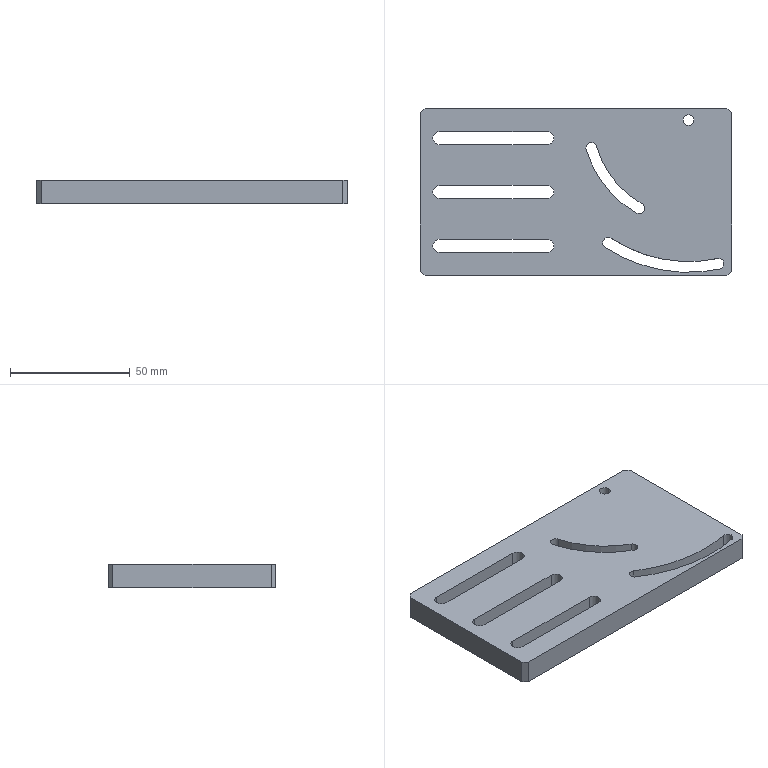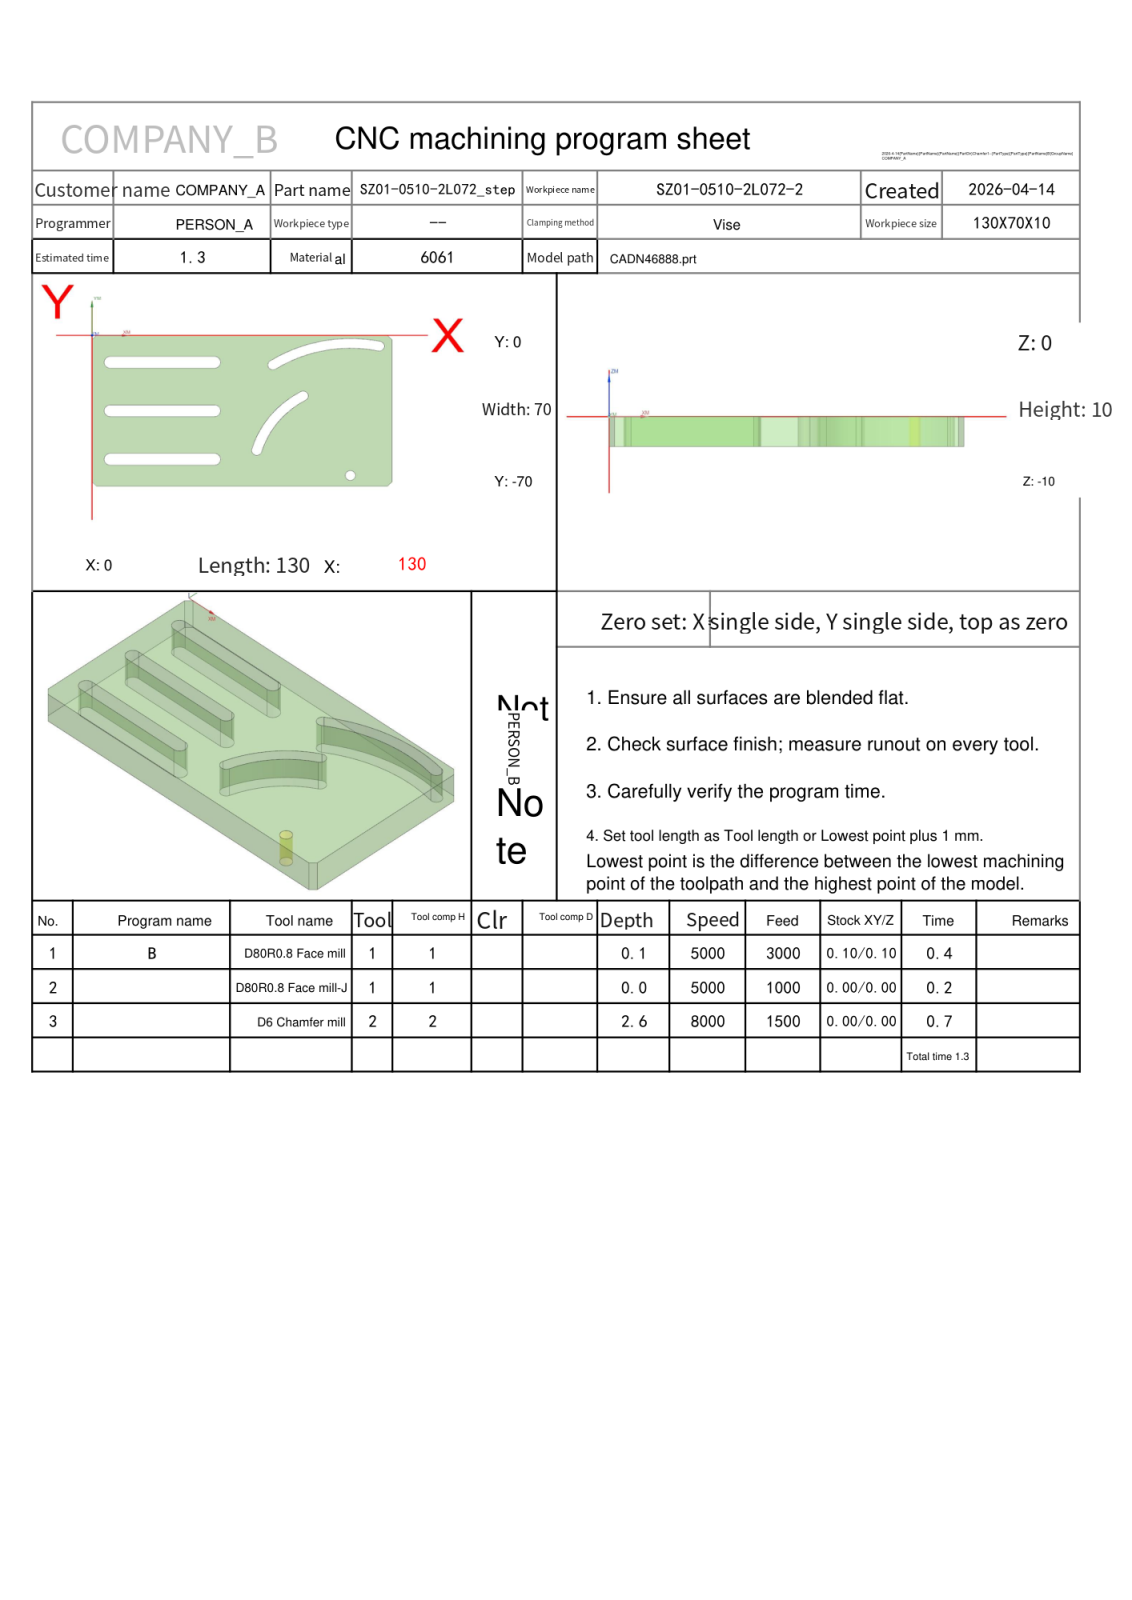NC program | NX | posted by the shop | part box 130 x 70 x 10 mm
Whole program:
%
O0001
(Machine time: 1.90 MIN)
(===Total Tool:2===)
(T1=D80R0.8 Face mill D=80.  R=0.8  D-  H01 Z=0.    )
(T2=D6 Chamfer mill   D=6.   R=0.   D-  H02 Z=-2.55 )
G80 G90 G17 G49 G40
G91 G28 Z0
M01
N1 T01 M06
(D80R0.8 Face mill  D=80. R=0.8 H=01 ce=0.10 di=0.10)
G00 G90 G54 X182.097 Y-35. M03 S5000
G43 H01 Z20.
M08
Z3.375
G01 Z1.375 F3000.
X170.097
X-40.097
X-52.097
Z3.375
G00 X182.097
Z2.95
G01 Z.95
X170.097
X-40.097
X-52.097
Z2.95
G00 X182.097
Z2.525
G01 Z.525
X170.097
X-40.097
X-52.097
Z2.525
G00 X182.097
Z2.1
G01 Z.1
X170.097
X-40.097
X-52.097
Z2.1
G00 Z20.
G91 G28 Z0.0
M05
M09
G91 G28 Z0.0
M01
N2 T01 M06
(D80R0.8 Face mill-J  D=80. R=0.8 H=01 ce=0.00 di=0.00)
G00 G90 G54 X181.999 Y-35. M03 S5000
G43 H01 Z20.
M08
Z2.
G01 Z0.0 F1000.
X169.999
X-39.999
X-51.999
Z2.
G00 Z20.
G91 G28 Z0.0
M05
M09
G91 G28 Z0.0
M01
N3 T02 M06
(D6 Chamfer mill  D=6. R=0. H=02 ce=0.00 di=0.00)
G00 G90 G54 X112. Y-65. M03 S8000
G43 H02 Z20.
M08
G98 G81 X112. Y-65. Z-2.55 R3. F1000.
G80
G00 Z20.
G00 G90 X64.614 Y1.227 M03 S6500
Z20.
Z.172
G01 Z-1.2 F1500.
G03 X64.9 Y1.027 I1.286 J1.532
G01 X64.946 Y.997
X65. Y1.
X128.
X128.259 Y.966
X128.5 Y.866
X128.707 Y.707
X130.707 Y-1.293
X130.866 Y-1.5
X130.966 Y-1.741
X131. Y-2.
Y-68.
X130.966 Y-68.259
X130.866 Y-68.5
X130.707 Y-68.707
X128.707 Y-70.707
X128.5 Y-70.866
X128.259 Y-70.966
X128. Y-71.
X2.
X1.741 Y-70.966
X1.5 Y-70.866
X1.293 Y-70.707
X-.707 Y-68.707
X-.866 Y-68.5
X-.966 Y-68.259
X-1. Y-68.
Y-2.
X-.966 Y-1.741
X-.866 Y-1.5
X-.707 Y-1.293
X1.293 Y.707
X1.5 Y.866
X1.741 Y.966
X2. Y1.
X65.
X65.054 Y.997
X65.1 Y1.027
G03 X65.386 Y1.227 I-1. J1.732
G01 Z.172
G00 Z10.
X113.065 Y-65.407
Z.294
G01 Z-1.2
G03 X113.234 Y-65.102 I-1.658 J1.118
G01 X113.259 Y-65.054
X113.25 Y-65.
G03 X112. Y-63.75 I-1.25 J0.0
X110.75 Y-65. I0.0 J-1.25
X112. Y-66.25 I1.25 J0.0
X113.223 Y-65.26 I0.0 J1.25
G01 X113.25 Y-65.
X113.259 Y-64.946
X113.234 Y-64.898
G03 X113.065 Y-64.593 I-1.827 J-.813
G01 Z.294
G00 Z10.
X78.375 Y-37.807
Z.189
G01 Z-1.2
G03 X78.042 Y-37.913 I.439 J-1.951
G01 X77.991 Y-37.932
X77.96 Y-37.977
G03 X70.21 Y-53.06 I34.04 J-27.023
X70.162 Y-53.403 I1.202 J-.343
X71.412 Y-54.653 I1.25 J0.0
X72.614 Y-53.747 I0.0 J1.25
G02 X92.107 Y-29.193 I39.386 J-11.253
G03 X92.75 Y-28.1 I-.607 J1.093
X91.5 Y-26.85 I-1.25 J0.0
X90.893 Y-27.007 I0.0 J-1.25
X77.96 Y-37.977 I21.107 J-37.993
G01 X77.924 Y-38.017
X77.917 Y-38.071
G03 X77.89 Y-38.403 I1.972 J-.333
G01 Y-38.418
Z.189
G00 Z10.
X100.778 Y-3.699
Z.188
G01 Z-1.2
G03 X100.458 Y-3.561 I-.947 J-1.762
G01 X100.407 Y-3.542
X100.355 Y-3.556
G03 X77.727 Y-12.689 I11.645 J-61.444
X77.162 Y-13.735 I.685 J-1.046
X78.412 Y-14.985 I1.25 J0.0
X79.097 Y-14.78 I0.0 J1.25
G02 X112. Y-4.962 I32.903 J-50.22
X124.245 Y-6.224 I0.0 J-60.038
G03 X124.5 Y-6.25 I.255 J1.224
X125.75 Y-5. I0.0 J1.25
X124.755 Y-3.776 I-1.25 J0.0
X112. Y-2.462 I-12.755 J-61.224
X100.355 Y-3.556 I0.0 J-62.538
G01 X100.301 Y-3.562
X100.261 Y-3.599
G03 X100.013 Y-3.844 I1.278 J-1.539
G01 Z.188
G00 Z10.
X30.886 Y-10.977
Z.172
G01 Z-1.2
G03 X30.6 Y-10.777 I-1.286 J-1.532
G01 X30.554 Y-10.747
X30.5 Y-10.75
X8.
G03 X6.25 Y-12.5 I0.0 J-1.75
X8. Y-14.25 I1.75 J0.0
G01 X53.
G03 X54.75 Y-12.5 I0.0 J1.75
X53. Y-10.75 I-1.75 J0.0
G01 X30.5
X30.446 Y-10.747
X30.4 Y-10.777
G03 X30.114 Y-10.977 I1. J-1.732
G01 Z.172
G00 Z10.
Y-36.523
Z.172
G01 Z-1.2
G03 X30.4 Y-36.723 I1.286 J1.532
G01 X30.446 Y-36.753
X30.5 Y-36.75
X53.
G03 X54.75 Y-35. I0.0 J1.75
X53. Y-33.25 I-1.75 J0.0
G01 X8.
G03 X6.25 Y-35. I0.0 J-1.75
X8. Y-36.75 I1.75 J0.0
G01 X30.5
X30.554 Y-36.753
X30.6 Y-36.723
G03 X30.886 Y-36.523 I-1. J1.732
G01 Z.172
G00 Z10.
X30.114 Y-59.023
Z.172
G01 Z-1.2
G03 X30.4 Y-59.223 I1.286 J1.532
G01 X30.446 Y-59.253
X30.5 Y-59.25
X53.
G03 X54.75 Y-57.5 I0.0 J1.75
X53. Y-55.75 I-1.75 J0.0
G01 X8.
G03 X6.25 Y-57.5 I0.0 J-1.75
X8. Y-59.25 I1.75 J0.0
G01 X30.5
X30.554 Y-59.253
X30.6 Y-59.223
G03 X30.886 Y-59.023 I-1. J1.732
G01 Z.172
G00 Z20.
M05
M09
G91 G28 Z0.0
G91 G28 Y0.0
M30
%